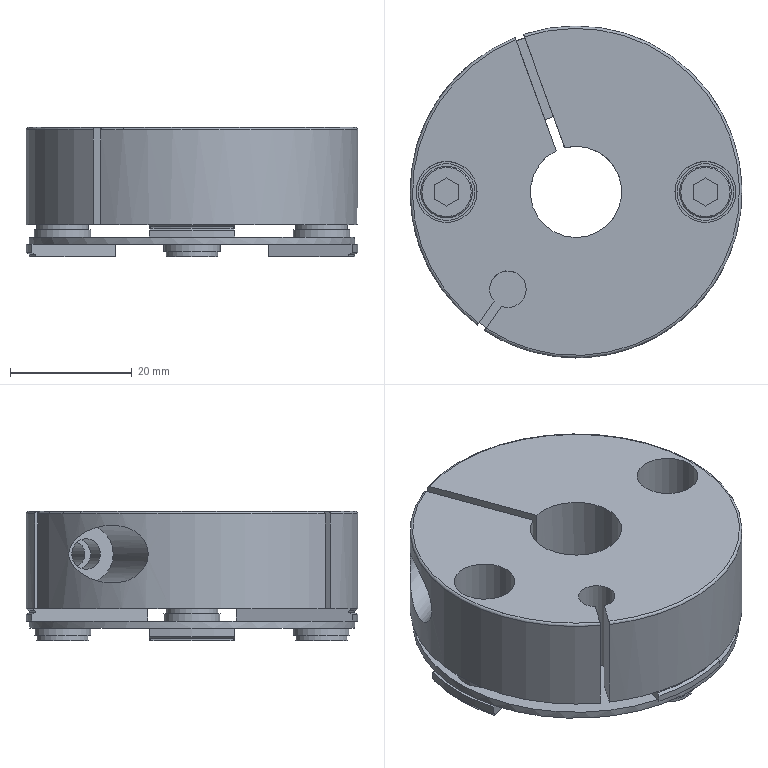Part | NX | features R_5003_007_C-SCPW55-12-15 2 | 1 solid | 89 faces | box 54.5 x 54.5 x 21.2 mm | volume 34124 mm3 | plane 52 | cylinder 23 | cone 8 | torus 6 | commonest cylinder face diameters 54.5 x6 8.5 x4 9.3 x4 10 x2 4.134 x1 5 x1